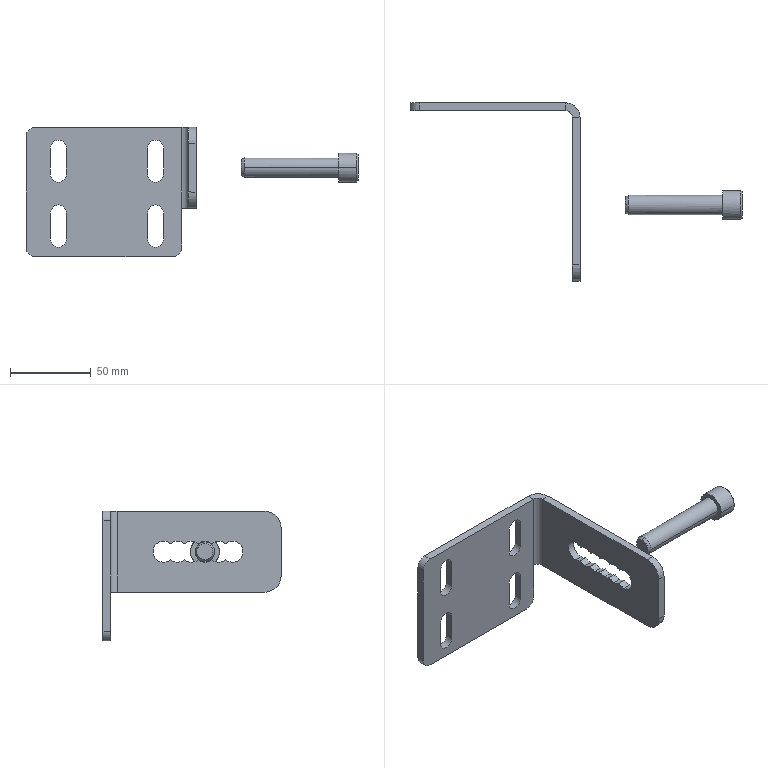Part | STEP file | BASE ACTIVACION BALANCIN | 2 solids | 76 faces | box 205 x 110 x 80 mm | volume 64247 mm3 | cylinder 41 | plane 31 | cone 4 | commonest cylinder face diameters 13 x18 10 x12 12 x5 17.8 x2 20 x2 8 x1